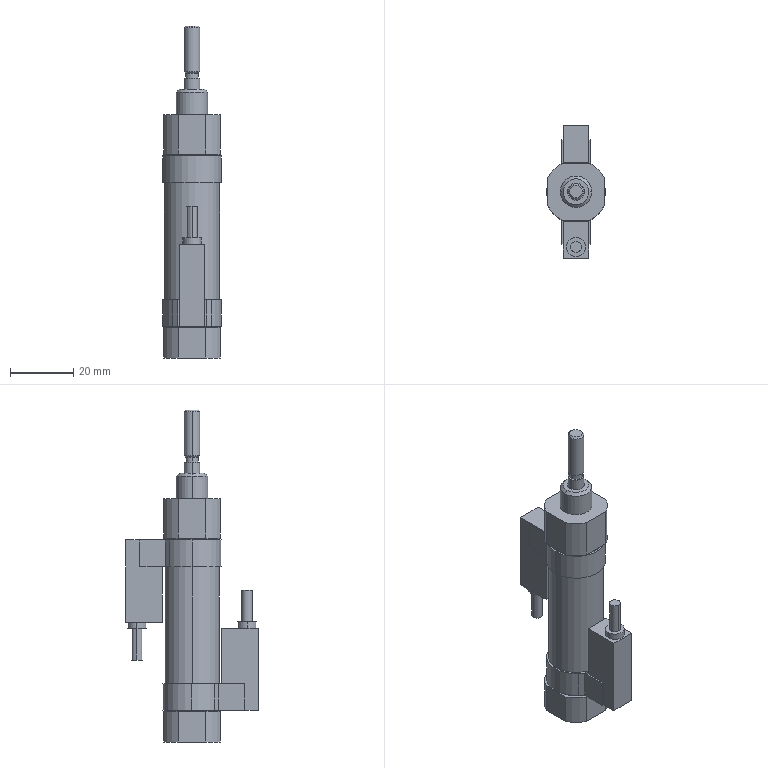Part | STEP file | Mount electronic clip sA_CDJ2B16-30-C73(0) | 3 solids | 113 faces | box 18.6 x 41.8 x 105 mm | volume 26366 mm3 | plane 53 | cylinder 46 | cone 10 | spline 4 | commonest cylinder face diameters 18.6 x8 20 x8 17.4 x6 3.4 x4 4.13 x4 5 x4